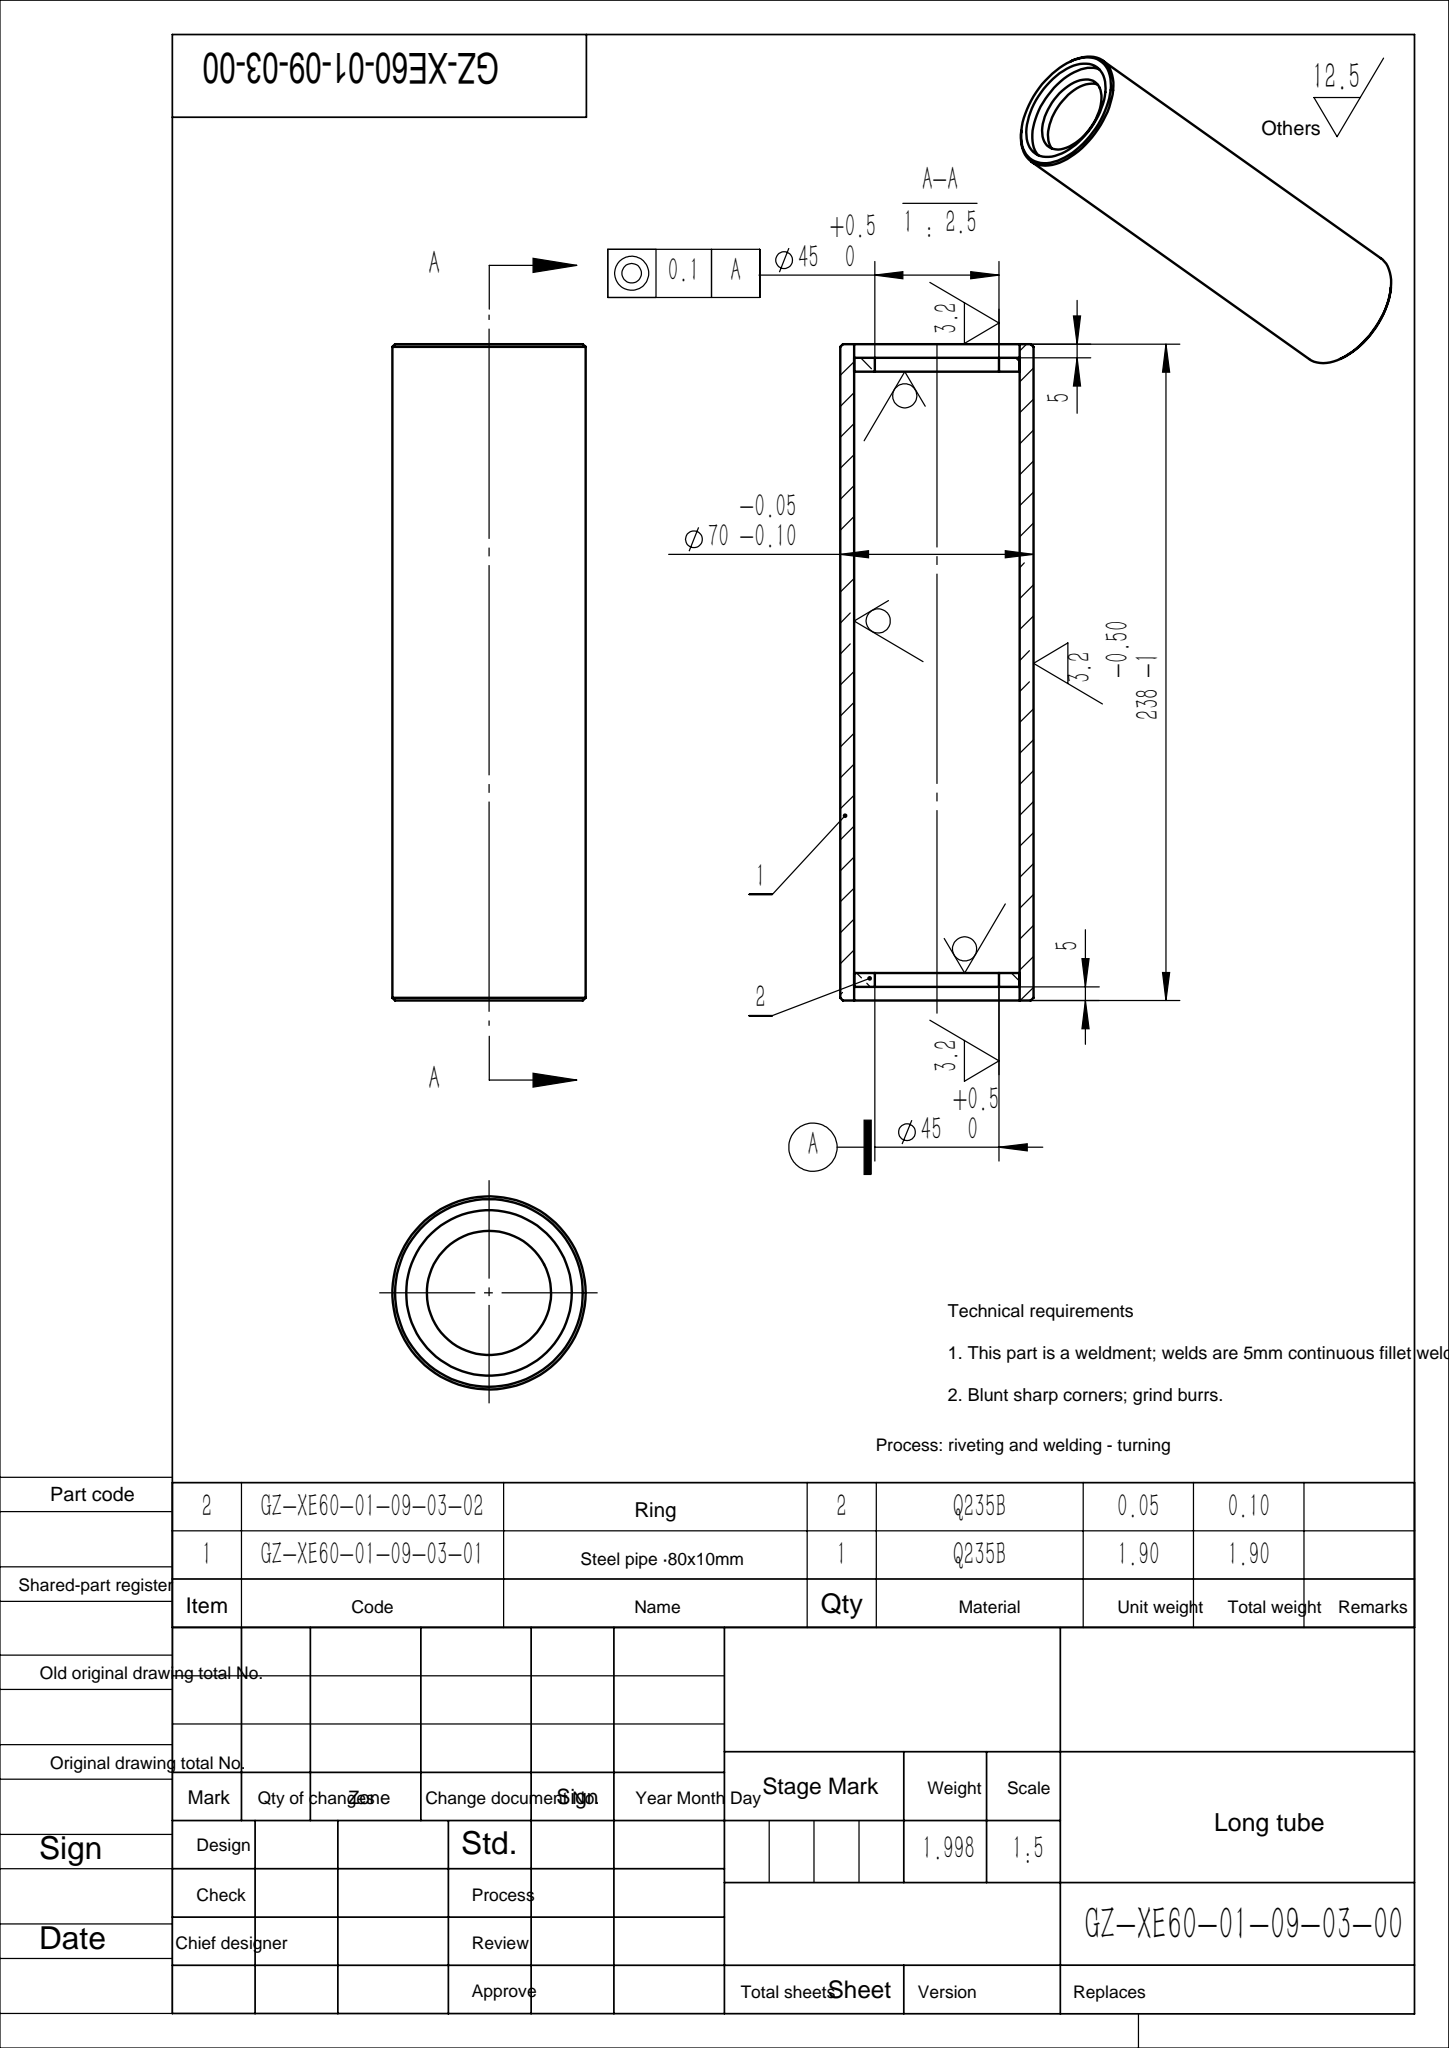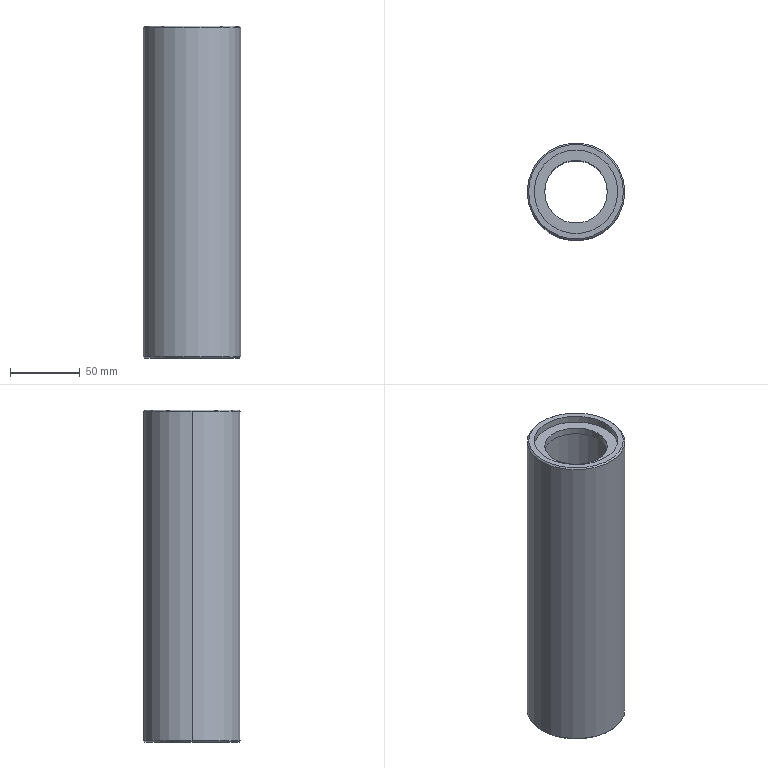Part | SolidWorks | 3 solids | 22 faces | box 70 x 70 x 238 mm | volume 255154 mm3 | cylinder 12 | plane 6 | cone 4 | commonest cylinder face diameters 60 x6 45 x4 70 x2